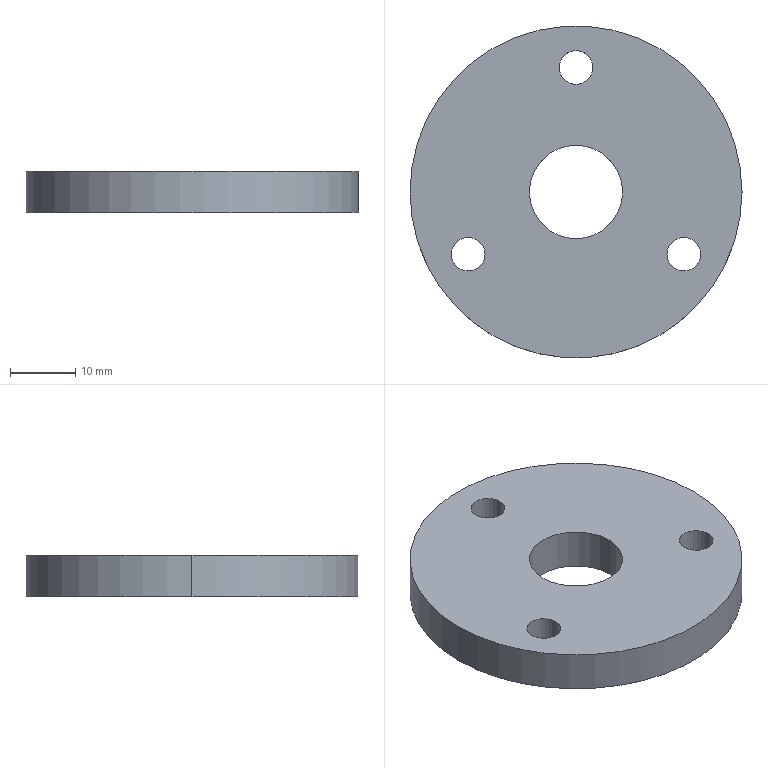Part | SolidWorks | features Extrusion 1, ICE 1 | 1 solid | 12 faces | box 50.8 x 50.8 x 6.35 mm | volume 11453 mm3 | cylinder 10 | plane 2 | commonest cylinder face diameters 5.156 x6 14.3 x2 50.8 x2
STEP:
#1=CARTESIAN_POINT('',(0.548,-0.375,-0.25));
#2=VERTEX_POINT('',#1);
#3=CARTESIAN_POINT('',(0.751,-0.375,-0.25));
#4=VERTEX_POINT('',#3);
#5=CARTESIAN_POINT('',(0.6495,-0.375,-0.25));
#6=DIRECTION('',(0.,0.,1.));
#7=DIRECTION('',(1.,0.,0.));
#8=AXIS2_PLACEMENT_3D('',#5,#6,#7);
#9=CIRCLE('',#8,0.1015);
#10=EDGE_CURVE('',#2,#4,#9,.T.);
#11=ORIENTED_EDGE('',*,*,#10,.F.);
#12=CARTESIAN_POINT('',(0.548,-0.375,0.));
#13=VERTEX_POINT('',#12);
#14=CARTESIAN_POINT('',(0.548,-0.375,-0.25));
#15=DIRECTION('',(0.,0.,1.));
#16=VECTOR('',#15,39.37);
#17=LINE('',#14,#16);
#18=EDGE_CURVE('',#2,#13,#17,.T.);
#19=ORIENTED_EDGE('',*,*,#18,.T.);
#20=CARTESIAN_POINT('',(0.751,-0.375,0.));
#21=VERTEX_POINT('',#20);
#22=CARTESIAN_POINT('',(0.6495,-0.375,0.));
#23=DIRECTION('',(0.,0.,1.));
#24=DIRECTION('',(1.,0.,0.));
#25=AXIS2_PLACEMENT_3D('',#22,#23,#24);
#26=CIRCLE('',#25,0.1015);
#27=EDGE_CURVE('',#13,#21,#26,.T.);
#28=ORIENTED_EDGE('',*,*,#27,.T.);
#29=CARTESIAN_POINT('',(0.751,-0.375,-0.25));
#30=DIRECTION('',(0.,0.,1.));
#31=VECTOR('',#30,39.37);
#32=LINE('',#29,#31);
#33=EDGE_CURVE('',#4,#21,#32,.T.);
#34=ORIENTED_EDGE('',*,*,#33,.F.);
#35=EDGE_LOOP('',(#11,#19,#28,#34));
#36=FACE_OUTER_BOUND('',#35,.T.);
#37=CARTESIAN_POINT('',(0.6495,-0.375,-0.25));
#38=DIRECTION('',(0.,0.,1.));
#39=DIRECTION('',(1.,0.,0.));
#40=AXIS2_PLACEMENT_3D('',#37,#38,#39);
#41=CYLINDRICAL_SURFACE('',#40,0.1015);
#42=ADVANCED_FACE('',(#36),#41,.F.);
#43=CARTESIAN_POINT('',(-0.751,-0.375,-0.25));
#44=VERTEX_POINT('',#43);
#45=CARTESIAN_POINT('',(-0.548,-0.375,-0.25));
#46=VERTEX_POINT('',#45);
#47=CARTESIAN_POINT('',(-0.6495,-0.375,-0.25));
#48=DIRECTION('',(0.,0.,1.));
#49=DIRECTION('',(1.,0.,0.));
#50=AXIS2_PLACEMENT_3D('',#47,#48,#49);
#51=CIRCLE('',#50,0.1015);
#52=EDGE_CURVE('',#44,#46,#51,.T.);
#53=ORIENTED_EDGE('',*,*,#52,.F.);
#54=CARTESIAN_POINT('',(-0.751,-0.375,0.));
#55=VERTEX_POINT('',#54);
#56=CARTESIAN_POINT('',(-0.751,-0.375,-0.25));
#57=DIRECTION('',(0.,0.,1.));
#58=VECTOR('',#57,39.37);
#59=LINE('',#56,#58);
#60=EDGE_CURVE('',#44,#55,#59,.T.);
#61=ORIENTED_EDGE('',*,*,#60,.T.);
#62=CARTESIAN_POINT('',(-0.548,-0.375,0.));
#63=VERTEX_POINT('',#62);
#64=CARTESIAN_POINT('',(-0.6495,-0.375,0.));
#65=DIRECTION('',(0.,0.,1.));
#66=DIRECTION('',(1.,0.,0.));
#67=AXIS2_PLACEMENT_3D('',#64,#65,#66);
#68=CIRCLE('',#67,0.1015);
#69=EDGE_CURVE('',#55,#63,#68,.T.);
#70=ORIENTED_EDGE('',*,*,#69,.T.);
#71=CARTESIAN_POINT('',(-0.548,-0.375,-0.25));
#72=DIRECTION('',(0.,0.,1.));
#73=VECTOR('',#72,39.37);
#74=LINE('',#71,#73);
#75=EDGE_CURVE('',#46,#63,#74,.T.);
#76=ORIENTED_EDGE('',*,*,#75,.F.);
#77=EDGE_LOOP('',(#53,#61,#70,#76));
#78=FACE_OUTER_BOUND('',#77,.T.);
#79=CARTESIAN_POINT('',(-0.6495,-0.375,-0.25));
#80=DIRECTION('',(0.,0.,1.));
#81=DIRECTION('',(1.,0.,0.));
#82=AXIS2_PLACEMENT_3D('',#79,#80,#81);
#83=CYLINDRICAL_SURFACE('',#82,0.1015);
#84=ADVANCED_FACE('',(#78),#83,.F.);
#85=CARTESIAN_POINT('',(-0.1015,0.75,-0.25));
#86=VERTEX_POINT('',#85);
#87=CARTESIAN_POINT('',(0.1015,0.75,-0.25));
#88=VERTEX_POINT('',#87);
#89=CARTESIAN_POINT('',(0.,0.75,-0.25));
#90=DIRECTION('',(0.,0.,1.));
#91=DIRECTION('',(1.,0.,0.));
#92=AXIS2_PLACEMENT_3D('',#89,#90,#91);
#93=CIRCLE('',#92,0.1015);
#94=EDGE_CURVE('',#86,#88,#93,.T.);
#95=ORIENTED_EDGE('',*,*,#94,.F.);
#96=CARTESIAN_POINT('',(-0.1015,0.75,0.));
#97=VERTEX_POINT('',#96);
#98=CARTESIAN_POINT('',(-0.1015,0.75,-0.25));
#99=DIRECTION('',(0.,0.,1.));
#100=VECTOR('',#99,39.37);
#101=LINE('',#98,#100);
#102=EDGE_CURVE('',#86,#97,#101,.T.);
#103=ORIENTED_EDGE('',*,*,#102,.T.);
#104=CARTESIAN_POINT('',(0.1015,0.75,0.));
#105=VERTEX_POINT('',#104);
#106=CARTESIAN_POINT('',(0.,0.75,0.));
#107=DIRECTION('',(0.,0.,1.));
#108=DIRECTION('',(1.,0.,0.));
#109=AXIS2_PLACEMENT_3D('',#106,#107,#108);
#110=CIRCLE('',#109,0.1015);
#111=EDGE_CURVE('',#97,#105,#110,.T.);
#112=ORIENTED_EDGE('',*,*,#111,.T.);
#113=CARTESIAN_POINT('',(0.1015,0.75,-0.25));
#114=DIRECTION('',(0.,0.,1.));
#115=VECTOR('',#114,39.37);
#116=LINE('',#113,#115);
#117=EDGE_CURVE('',#88,#105,#116,.T.);
#118=ORIENTED_EDGE('',*,*,#117,.F.);
#119=EDGE_LOOP('',(#95,#103,#112,#118));
#120=FACE_OUTER_BOUND('',#119,.T.);
#121=CARTESIAN_POINT('',(0.,0.75,-0.25));
#122=DIRECTION('',(0.,0.,1.));
#123=DIRECTION('',(1.,0.,0.));
#124=AXIS2_PLACEMENT_3D('',#121,#122,#123);
#125=CYLINDRICAL_SURFACE('',#124,0.1015);
#126=ADVANCED_FACE('',(#120),#125,.F.);
#127=CARTESIAN_POINT('',(-0.2815,0.,-0.25));
#128=VERTEX_POINT('',#127);
#129=CARTESIAN_POINT('',(0.2815,0.,-0.25));
#130=VERTEX_POINT('',#129);
#131=CARTESIAN_POINT('',(0.,0.,-0.25));
#132=DIRECTION('',(0.,0.,1.));
#133=DIRECTION('',(1.,0.,0.));
#134=AXIS2_PLACEMENT_3D('',#131,#132,#133);
#135=CIRCLE('',#134,0.2815);
#136=EDGE_CURVE('',#128,#130,#135,.T.);
#137=ORIENTED_EDGE('',*,*,#136,.F.);
#138=CARTESIAN_POINT('',(-0.2815,0.,0.));
#139=VERTEX_POINT('',#138);
#140=CARTESIAN_POINT('',(-0.2815,0.,-0.25));
#141=DIRECTION('',(0.,0.,1.));
#142=VECTOR('',#141,39.37);
#143=LINE('',#140,#142);
#144=EDGE_CURVE('',#128,#139,#143,.T.);
#145=ORIENTED_EDGE('',*,*,#144,.T.);
#146=CARTESIAN_POINT('',(0.2815,0.,0.));
#147=VERTEX_POINT('',#146);
#148=CARTESIAN_POINT('',(0.,0.,0.));
#149=DIRECTION('',(0.,0.,1.));
#150=DIRECTION('',(1.,0.,0.));
#151=AXIS2_PLACEMENT_3D('',#148,#149,#150);
#152=CIRCLE('',#151,0.2815);
#153=EDGE_CURVE('',#139,#147,#152,.T.);
#154=ORIENTED_EDGE('',*,*,#153,.T.);
#155=CARTESIAN_POINT('',(0.2815,0.,-0.25));
#156=DIRECTION('',(0.,0.,1.));
#157=VECTOR('',#156,39.37);
#158=LINE('',#155,#157);
#159=EDGE_CURVE('',#130,#147,#158,.T.);
#160=ORIENTED_EDGE('',*,*,#159,.F.);
#161=EDGE_LOOP('',(#137,#145,#154,#160));
#162=FACE_OUTER_BOUND('',#161,.T.);
#163=CARTESIAN_POINT('',(0.,0.,-0.25));
#164=DIRECTION('',(0.,0.,1.));
#165=DIRECTION('',(1.,0.,0.));
#166=AXIS2_PLACEMENT_3D('',#163,#164,#165);
#167=CYLINDRICAL_SURFACE('',#166,0.2815);
#168=ADVANCED_FACE('',(#162),#167,.F.);
#169=CARTESIAN_POINT('',(1.,0.,-0.25));
#170=VERTEX_POINT('',#169);
#171=CARTESIAN_POINT('',(-1.,0.,-0.25));
#172=VERTEX_POINT('',#171);
#173=CARTESIAN_POINT('',(0.,0.,-0.25));
#174=DIRECTION('',(0.,0.,1.));
#175=DIRECTION('',(1.,0.,0.));
#176=AXIS2_PLACEMENT_3D('',#173,#174,#175);
#177=CIRCLE('',#176,1.);
#178=EDGE_CURVE('',#170,#172,#177,.T.);
#179=ORIENTED_EDGE('',*,*,#178,.T.);
#180=CARTESIAN_POINT('',(-1.,0.,0.));
#181=VERTEX_POINT('',#180);
#182=CARTESIAN_POINT('',(-1.,0.,-0.25));
#183=DIRECTION('',(0.,0.,1.));
#184=VECTOR('',#183,39.37);
#185=LINE('',#182,#184);
#186=EDGE_CURVE('',#172,#181,#185,.T.);
#187=ORIENTED_EDGE('',*,*,#186,.T.);
#188=CARTESIAN_POINT('',(1.,0.,0.));
#189=VERTEX_POINT('',#188);
#190=CARTESIAN_POINT('',(0.,0.,0.));
#191=DIRECTION('',(0.,0.,1.));
#192=DIRECTION('',(1.,0.,0.));
#193=AXIS2_PLACEMENT_3D('',#190,#191,#192);
#194=CIRCLE('',#193,1.);
#195=EDGE_CURVE('',#189,#181,#194,.T.);
#196=ORIENTED_EDGE('',*,*,#195,.F.);
#197=CARTESIAN_POINT('',(1.,0.,-0.25));
#198=DIRECTION('',(0.,0.,1.));
#199=VECTOR('',#198,39.37);
#200=LINE('',#197,#199);
#201=EDGE_CURVE('',#170,#189,#200,.T.);
#202=ORIENTED_EDGE('',*,*,#201,.F.);
#203=EDGE_LOOP('',(#179,#187,#196,#202));
#204=FACE_OUTER_BOUND('',#203,.T.);
#205=CARTESIAN_POINT('',(0.,0.,-0.25));
#206=DIRECTION('',(0.,0.,1.));
#207=DIRECTION('',(1.,0.,0.));
#208=AXIS2_PLACEMENT_3D('',#205,#206,#207);
#209=CYLINDRICAL_SURFACE('',#208,1.);
#210=ADVANCED_FACE('',(#204),#209,.T.);
#211=ORIENTED_EDGE('',*,*,#186,.F.);
#212=CARTESIAN_POINT('',(0.,0.,-0.25));
#213=DIRECTION('',(0.,0.,1.));
#214=DIRECTION('',(1.,0.,0.));
#215=AXIS2_PLACEMENT_3D('',#212,#213,#214);
#216=CIRCLE('',#215,1.);
#217=EDGE_CURVE('',#172,#170,#216,.T.);
#218=ORIENTED_EDGE('',*,*,#217,.T.);
#219=ORIENTED_EDGE('',*,*,#201,.T.);
#220=CARTESIAN_POINT('',(0.,0.,0.));
#221=DIRECTION('',(0.,0.,1.));
#222=DIRECTION('',(1.,0.,0.));
#223=AXIS2_PLACEMENT_3D('',#220,#221,#222);
#224=CIRCLE('',#223,1.);
#225=EDGE_CURVE('',#181,#189,#224,.T.);
#226=ORIENTED_EDGE('',*,*,#225,.F.);
#227=EDGE_LOOP('',(#211,#218,#219,#226));
#228=FACE_OUTER_BOUND('',#227,.T.);
#229=CARTESIAN_POINT('',(0.,0.,-0.25));
#230=DIRECTION('',(0.,0.,1.));
#231=DIRECTION('',(1.,0.,0.));
#232=AXIS2_PLACEMENT_3D('',#229,#230,#231);
#233=CYLINDRICAL_SURFACE('',#232,1.);
#234=ADVANCED_FACE('',(#228),#233,.T.);
#235=CARTESIAN_POINT('',(0.6495,-0.375,-0.25));
#236=DIRECTION('',(0.,0.,1.));
#237=DIRECTION('',(1.,0.,0.));
#238=AXIS2_PLACEMENT_3D('',#235,#236,#237);
#239=CIRCLE('',#238,0.1015);
#240=EDGE_CURVE('',#4,#2,#239,.T.);
#241=ORIENTED_EDGE('',*,*,#240,.T.);
#242=ORIENTED_EDGE('',*,*,#10,.T.);
#243=EDGE_LOOP('',(#241,#242));
#244=FACE_BOUND('',#243,.T.);
#245=CARTESIAN_POINT('',(-0.6495,-0.375,-0.25));
#246=DIRECTION('',(0.,0.,1.));
#247=DIRECTION('',(1.,0.,0.));
#248=AXIS2_PLACEMENT_3D('',#245,#246,#247);
#249=CIRCLE('',#248,0.1015);
#250=EDGE_CURVE('',#46,#44,#249,.T.);
#251=ORIENTED_EDGE('',*,*,#250,.T.);
#252=ORIENTED_EDGE('',*,*,#52,.T.);
#253=EDGE_LOOP('',(#251,#252));
#254=FACE_BOUND('',#253,.T.);
#255=CARTESIAN_POINT('',(0.,0.75,-0.25));
#256=DIRECTION('',(0.,0.,1.));
#257=DIRECTION('',(1.,0.,0.));
#258=AXIS2_PLACEMENT_3D('',#255,#256,#257);
#259=CIRCLE('',#258,0.1015);
#260=EDGE_CURVE('',#88,#86,#259,.T.);
#261=ORIENTED_EDGE('',*,*,#260,.T.);
#262=ORIENTED_EDGE('',*,*,#94,.T.);
#263=EDGE_LOOP('',(#261,#262));
#264=FACE_BOUND('',#263,.T.);
#265=CARTESIAN_POINT('',(0.,0.,-0.25));
#266=DIRECTION('',(0.,0.,1.));
#267=DIRECTION('',(1.,0.,0.));
#268=AXIS2_PLACEMENT_3D('',#265,#266,#267);
#269=CIRCLE('',#268,0.2815);
#270=EDGE_CURVE('',#130,#128,#269,.T.);
#271=ORIENTED_EDGE('',*,*,#270,.T.);
#272=ORIENTED_EDGE('',*,*,#136,.T.);
#273=EDGE_LOOP('',(#271,#272));
#274=FACE_BOUND('',#273,.T.);
#275=ORIENTED_EDGE('',*,*,#178,.F.);
#276=ORIENTED_EDGE('',*,*,#217,.F.);
#277=EDGE_LOOP('',(#275,#276));
#278=FACE_OUTER_BOUND('',#277,.T.);
#279=CARTESIAN_POINT('',(0.,0.,-0.25));
#280=DIRECTION('',(0.,0.,1.));
#281=DIRECTION('',(1.,0.,0.));
#282=AXIS2_PLACEMENT_3D('',#279,#280,#281);
#283=PLANE('',#282);
#284=ADVANCED_FACE('',(#244,#254,#264,#274,#278),#283,.F.);
#285=CARTESIAN_POINT('',(0.6495,-0.375,0.));
#286=DIRECTION('',(0.,0.,1.));
#287=DIRECTION('',(1.,0.,0.));
#288=AXIS2_PLACEMENT_3D('',#285,#286,#287);
#289=CIRCLE('',#288,0.1015);
#290=EDGE_CURVE('',#21,#13,#289,.T.);
#291=ORIENTED_EDGE('',*,*,#290,.F.);
#292=ORIENTED_EDGE('',*,*,#27,.F.);
#293=EDGE_LOOP('',(#291,#292));
#294=FACE_BOUND('',#293,.T.);
#295=CARTESIAN_POINT('',(-0.6495,-0.375,0.));
#296=DIRECTION('',(0.,0.,1.));
#297=DIRECTION('',(1.,0.,0.));
#298=AXIS2_PLACEMENT_3D('',#295,#296,#297);
#299=CIRCLE('',#298,0.1015);
#300=EDGE_CURVE('',#63,#55,#299,.T.);
#301=ORIENTED_EDGE('',*,*,#300,.F.);
#302=ORIENTED_EDGE('',*,*,#69,.F.);
#303=EDGE_LOOP('',(#301,#302));
#304=FACE_BOUND('',#303,.T.);
#305=CARTESIAN_POINT('',(0.,0.75,0.));
#306=DIRECTION('',(0.,0.,1.));
#307=DIRECTION('',(1.,0.,0.));
#308=AXIS2_PLACEMENT_3D('',#305,#306,#307);
#309=CIRCLE('',#308,0.1015);
#310=EDGE_CURVE('',#105,#97,#309,.T.);
#311=ORIENTED_EDGE('',*,*,#310,.F.);
#312=ORIENTED_EDGE('',*,*,#111,.F.);
#313=EDGE_LOOP('',(#311,#312));
#314=FACE_BOUND('',#313,.T.);
#315=CARTESIAN_POINT('',(0.,0.,0.));
#316=DIRECTION('',(0.,0.,1.));
#317=DIRECTION('',(1.,0.,0.));
#318=AXIS2_PLACEMENT_3D('',#315,#316,#317);
#319=CIRCLE('',#318,0.2815);
#320=EDGE_CURVE('',#147,#139,#319,.T.);
#321=ORIENTED_EDGE('',*,*,#320,.F.);
#322=ORIENTED_EDGE('',*,*,#153,.F.);
#323=EDGE_LOOP('',(#321,#322));
#324=FACE_BOUND('',#323,.T.);
#325=ORIENTED_EDGE('',*,*,#195,.T.);
#326=ORIENTED_EDGE('',*,*,#225,.T.);
#327=EDGE_LOOP('',(#325,#326));
#328=FACE_OUTER_BOUND('',#327,.T.);
#329=CARTESIAN_POINT('',(0.,0.,0.));
#330=DIRECTION('',(0.,0.,1.));
#331=DIRECTION('',(1.,0.,0.));
#332=AXIS2_PLACEMENT_3D('',#329,#330,#331);
#333=PLANE('',#332);
#334=ADVANCED_FACE('',(#294,#304,#314,#324,#328),#333,.T.);
#335=ORIENTED_EDGE('',*,*,#144,.F.);
#336=ORIENTED_EDGE('',*,*,#270,.F.);
#337=ORIENTED_EDGE('',*,*,#159,.T.);
#338=ORIENTED_EDGE('',*,*,#320,.T.);
#339=EDGE_LOOP('',(#335,#336,#337,#338));
#340=FACE_OUTER_BOUND('',#339,.T.);
#341=CARTESIAN_POINT('',(0.,0.,-0.25));
#342=DIRECTION('',(0.,0.,1.));
#343=DIRECTION('',(1.,0.,0.));
#344=AXIS2_PLACEMENT_3D('',#341,#342,#343);
#345=CYLINDRICAL_SURFACE('',#344,0.2815);
#346=ADVANCED_FACE('',(#340),#345,.F.);
#347=ORIENTED_EDGE('',*,*,#102,.F.);
#348=ORIENTED_EDGE('',*,*,#260,.F.);
#349=ORIENTED_EDGE('',*,*,#117,.T.);
#350=ORIENTED_EDGE('',*,*,#310,.T.);
#351=EDGE_LOOP('',(#347,#348,#349,#350));
#352=FACE_OUTER_BOUND('',#351,.T.);
#353=CARTESIAN_POINT('',(0.,0.75,-0.25));
#354=DIRECTION('',(0.,0.,1.));
#355=DIRECTION('',(1.,0.,0.));
#356=AXIS2_PLACEMENT_3D('',#353,#354,#355);
#357=CYLINDRICAL_SURFACE('',#356,0.1015);
#358=ADVANCED_FACE('',(#352),#357,.F.);
#359=ORIENTED_EDGE('',*,*,#60,.F.);
#360=ORIENTED_EDGE('',*,*,#250,.F.);
#361=ORIENTED_EDGE('',*,*,#75,.T.);
#362=ORIENTED_EDGE('',*,*,#300,.T.);
#363=EDGE_LOOP('',(#359,#360,#361,#362));
#364=FACE_OUTER_BOUND('',#363,.T.);
#365=CARTESIAN_POINT('',(-0.6495,-0.375,-0.25));
#366=DIRECTION('',(0.,0.,1.));
#367=DIRECTION('',(1.,0.,0.));
#368=AXIS2_PLACEMENT_3D('',#365,#366,#367);
#369=CYLINDRICAL_SURFACE('',#368,0.1015);
#370=ADVANCED_FACE('',(#364),#369,.F.);
#371=ORIENTED_EDGE('',*,*,#18,.F.);
#372=ORIENTED_EDGE('',*,*,#240,.F.);
#373=ORIENTED_EDGE('',*,*,#33,.T.);
#374=ORIENTED_EDGE('',*,*,#290,.T.);
#375=EDGE_LOOP('',(#371,#372,#373,#374));
#376=FACE_OUTER_BOUND('',#375,.T.);
#377=CARTESIAN_POINT('',(0.6495,-0.375,-0.25));
#378=DIRECTION('',(0.,0.,1.));
#379=DIRECTION('',(1.,0.,0.));
#380=AXIS2_PLACEMENT_3D('',#377,#378,#379);
#381=CYLINDRICAL_SURFACE('',#380,0.1015);
#382=ADVANCED_FACE('',(#376),#381,.F.);
#383=CLOSED_SHELL('',(#42,#84,#126,#168,#210,#234,#284,#334,#346,#358,#370,#382));
#384=MANIFOLD_SOLID_BREP('',#383);
#385=CARTESIAN_POINT('',(0.,0.,0.));
#386=DIRECTION('',(0.,0.,1.));
#387=DIRECTION('',(1.,0.,0.));
#388=AXIS2_PLACEMENT_3D('',#385,#386,#387);
#389=(LENGTH_UNIT()NAMED_UNIT(*)SI_UNIT($,.METRE.));
#390=LENGTH_MEASURE_WITH_UNIT(LENGTH_MEASURE(0.0254),#389);
#391=DIMENSIONAL_EXPONENTS(1.,0.,0.,0.,0.,0.,0.);
#392=(CONVERSION_BASED_UNIT('INCH',#390)LENGTH_UNIT()NAMED_UNIT(#391));
#393=UNCERTAINTY_MEASURE_WITH_UNIT(LENGTH_MEASURE(0.00001),#392,'','');
#394=(NAMED_UNIT(*)PLANE_ANGLE_UNIT()SI_UNIT($,.RADIAN.));
#395=(NAMED_UNIT(*)SI_UNIT($,.STERADIAN.)SOLID_ANGLE_UNIT());
#396=(GEOMETRIC_REPRESENTATION_CONTEXT(3)GLOBAL_UNCERTAINTY_ASSIGNED_CONTEXT((#393))GLOBAL_UNIT_ASSIGNED_CONTEXT((#392,#394,#395))REPRESENTATION_CONTEXT('',''));
#397=ADVANCED_BREP_SHAPE_REPRESENTATION('',(#384,#388),#396);